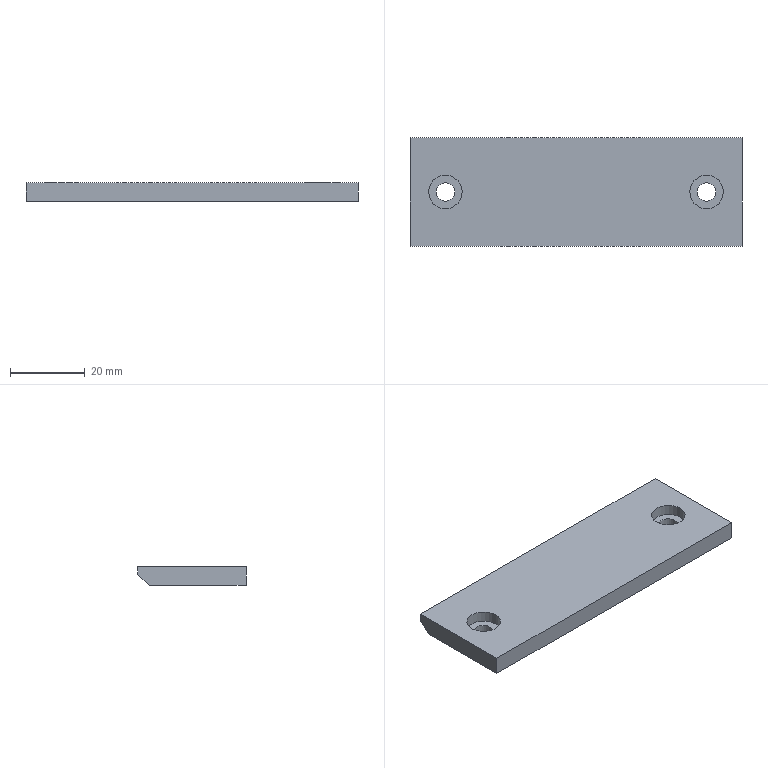Part | NX | features DATUM_CSYS 3, EXTRUDE 3, SKETCH 2 | 1 solid | 13 faces | box 89 x 29 x 5 mm | volume 12044 mm3 | plane 9 | cylinder 4 | commonest cylinder face diameters 5 x2 9 x2
STEP:
#1=CARTESIAN_POINT('',(0.,26.,0.));
#2=VERTEX_POINT('',#1);
#3=CARTESIAN_POINT('',(0.,29.,3.));
#4=VERTEX_POINT('',#3);
#5=CARTESIAN_POINT('',(0.,26.,0.));
#6=DIRECTION('',(0.,0.7071,0.7071));
#7=VECTOR('',#6,1000.);
#8=LINE('',#5,#7);
#9=EDGE_CURVE('',#2,#4,#8,.T.);
#10=ORIENTED_EDGE('',*,*,#9,.F.);
#11=CARTESIAN_POINT('',(0.,0.,0.));
#12=VERTEX_POINT('',#11);
#13=CARTESIAN_POINT('',(0.,29.,0.));
#14=DIRECTION('',(0.,-1.,0.));
#15=VECTOR('',#14,1000.);
#16=LINE('',#13,#15);
#17=EDGE_CURVE('',#2,#12,#16,.T.);
#18=ORIENTED_EDGE('',*,*,#17,.T.);
#19=CARTESIAN_POINT('',(0.,0.,5.));
#20=VERTEX_POINT('',#19);
#21=CARTESIAN_POINT('',(0.,0.,5.));
#22=DIRECTION('',(0.,0.,-1.));
#23=VECTOR('',#22,1000.);
#24=LINE('',#21,#23);
#25=EDGE_CURVE('',#20,#12,#24,.T.);
#26=ORIENTED_EDGE('',*,*,#25,.F.);
#27=CARTESIAN_POINT('',(0.,29.,5.));
#28=VERTEX_POINT('',#27);
#29=CARTESIAN_POINT('',(0.,29.,5.));
#30=DIRECTION('',(0.,-1.,0.));
#31=VECTOR('',#30,1000.);
#32=LINE('',#29,#31);
#33=EDGE_CURVE('',#28,#20,#32,.T.);
#34=ORIENTED_EDGE('',*,*,#33,.F.);
#35=CARTESIAN_POINT('',(0.,29.,5.));
#36=DIRECTION('',(0.,0.,-1.));
#37=VECTOR('',#36,1000.);
#38=LINE('',#35,#37);
#39=EDGE_CURVE('',#28,#4,#38,.T.);
#40=ORIENTED_EDGE('',*,*,#39,.T.);
#41=EDGE_LOOP('',(#10,#18,#26,#34,#40));
#42=FACE_BOUND('',#41,.T.);
#43=CARTESIAN_POINT('',(0.,29.,5.));
#44=DIRECTION('',(1.,0.,0.));
#45=DIRECTION('',(0.,0.,-1.));
#46=AXIS2_PLACEMENT_3D('',#43,#44,#45);
#47=PLANE('',#46);
#48=ADVANCED_FACE('',(#42),#47,.F.);
#49=CARTESIAN_POINT('',(75.,14.5,5.));
#50=VERTEX_POINT('',#49);
#51=CARTESIAN_POINT('',(79.5,14.5,5.));
#52=DIRECTION('',(0.,0.,-1.));
#53=DIRECTION('',(-1.,0.,0.));
#54=AXIS2_PLACEMENT_3D('',#51,#52,#53);
#55=CIRCLE('',#54,4.5);
#56=EDGE_CURVE('',#50,#50,#55,.T.);
#57=ORIENTED_EDGE('',*,*,#56,.F.);
#58=EDGE_LOOP('',(#57));
#59=FACE_BOUND('',#58,.T.);
#60=CARTESIAN_POINT('',(75.,14.5,2.));
#61=VERTEX_POINT('',#60);
#62=CARTESIAN_POINT('',(79.5,14.5,2.));
#63=DIRECTION('',(0.,0.,-1.));
#64=DIRECTION('',(-1.,0.,0.));
#65=AXIS2_PLACEMENT_3D('',#62,#63,#64);
#66=CIRCLE('',#65,4.5);
#67=EDGE_CURVE('',#61,#61,#66,.F.);
#68=ORIENTED_EDGE('',*,*,#67,.F.);
#69=EDGE_LOOP('',(#68));
#70=FACE_BOUND('',#69,.T.);
#71=CARTESIAN_POINT('',(79.5,14.5,5.));
#72=DIRECTION('',(0.,0.,-1.));
#73=DIRECTION('',(-1.,0.,0.));
#74=AXIS2_PLACEMENT_3D('',#71,#72,#73);
#75=CYLINDRICAL_SURFACE('',#74,4.5);
#76=ADVANCED_FACE('',(#59,#70),#75,.F.);
#77=CARTESIAN_POINT('',(89.,0.,0.));
#78=VERTEX_POINT('',#77);
#79=CARTESIAN_POINT('',(0.,0.,0.));
#80=DIRECTION('',(1.,0.,0.));
#81=VECTOR('',#80,1000.);
#82=LINE('',#79,#81);
#83=EDGE_CURVE('',#12,#78,#82,.T.);
#84=ORIENTED_EDGE('',*,*,#83,.T.);
#85=CARTESIAN_POINT('',(89.,0.,5.));
#86=VERTEX_POINT('',#85);
#87=CARTESIAN_POINT('',(89.,0.,5.));
#88=DIRECTION('',(0.,0.,-1.));
#89=VECTOR('',#88,1000.);
#90=LINE('',#87,#89);
#91=EDGE_CURVE('',#86,#78,#90,.T.);
#92=ORIENTED_EDGE('',*,*,#91,.F.);
#93=CARTESIAN_POINT('',(0.,0.,5.));
#94=DIRECTION('',(1.,0.,0.));
#95=VECTOR('',#94,1000.);
#96=LINE('',#93,#95);
#97=EDGE_CURVE('',#20,#86,#96,.T.);
#98=ORIENTED_EDGE('',*,*,#97,.F.);
#99=ORIENTED_EDGE('',*,*,#25,.T.);
#100=EDGE_LOOP('',(#84,#92,#98,#99));
#101=FACE_BOUND('',#100,.T.);
#102=CARTESIAN_POINT('',(0.,0.,5.));
#103=DIRECTION('',(0.,1.,0.));
#104=DIRECTION('',(0.,0.,1.));
#105=AXIS2_PLACEMENT_3D('',#102,#103,#104);
#106=PLANE('',#105);
#107=ADVANCED_FACE('',(#101),#106,.F.);
#108=CARTESIAN_POINT('',(89.,26.,0.));
#109=VERTEX_POINT('',#108);
#110=CARTESIAN_POINT('',(89.,0.,0.));
#111=DIRECTION('',(0.,1.,0.));
#112=VECTOR('',#111,1000.);
#113=LINE('',#110,#112);
#114=EDGE_CURVE('',#78,#109,#113,.T.);
#115=ORIENTED_EDGE('',*,*,#114,.T.);
#116=CARTESIAN_POINT('',(89.,29.,3.));
#117=VERTEX_POINT('',#116);
#118=CARTESIAN_POINT('',(89.,15.5,-10.5));
#119=DIRECTION('',(0.,0.7071,0.7071));
#120=VECTOR('',#119,1000.);
#121=LINE('',#118,#120);
#122=EDGE_CURVE('',#109,#117,#121,.T.);
#123=ORIENTED_EDGE('',*,*,#122,.T.);
#124=CARTESIAN_POINT('',(89.,29.,5.));
#125=VERTEX_POINT('',#124);
#126=CARTESIAN_POINT('',(89.,29.,5.));
#127=DIRECTION('',(0.,0.,-1.));
#128=VECTOR('',#127,1000.);
#129=LINE('',#126,#128);
#130=EDGE_CURVE('',#125,#117,#129,.T.);
#131=ORIENTED_EDGE('',*,*,#130,.F.);
#132=CARTESIAN_POINT('',(89.,0.,5.));
#133=DIRECTION('',(0.,1.,0.));
#134=VECTOR('',#133,1000.);
#135=LINE('',#132,#134);
#136=EDGE_CURVE('',#86,#125,#135,.T.);
#137=ORIENTED_EDGE('',*,*,#136,.F.);
#138=ORIENTED_EDGE('',*,*,#91,.T.);
#139=EDGE_LOOP('',(#115,#123,#131,#137,#138));
#140=FACE_BOUND('',#139,.T.);
#141=CARTESIAN_POINT('',(89.,0.,5.));
#142=DIRECTION('',(-1.,0.,0.));
#143=DIRECTION('',(0.,0.,1.));
#144=AXIS2_PLACEMENT_3D('',#141,#142,#143);
#145=PLANE('',#144);
#146=ADVANCED_FACE('',(#140),#145,.F.);
#147=ORIENTED_EDGE('',*,*,#130,.T.);
#148=CARTESIAN_POINT('',(55000.,29.,3.));
#149=DIRECTION('',(-1.,0.,0.));
#150=VECTOR('',#149,1000.);
#151=LINE('',#148,#150);
#152=EDGE_CURVE('',#117,#4,#151,.T.);
#153=ORIENTED_EDGE('',*,*,#152,.T.);
#154=ORIENTED_EDGE('',*,*,#39,.F.);
#155=CARTESIAN_POINT('',(89.,29.,5.));
#156=DIRECTION('',(-1.,0.,0.));
#157=VECTOR('',#156,1000.);
#158=LINE('',#155,#157);
#159=EDGE_CURVE('',#125,#28,#158,.T.);
#160=ORIENTED_EDGE('',*,*,#159,.F.);
#161=EDGE_LOOP('',(#147,#153,#154,#160));
#162=FACE_BOUND('',#161,.T.);
#163=CARTESIAN_POINT('',(89.,29.,5.));
#164=DIRECTION('',(0.,-1.,0.));
#165=DIRECTION('',(1.,0.,0.));
#166=AXIS2_PLACEMENT_3D('',#163,#164,#165);
#167=PLANE('',#166);
#168=ADVANCED_FACE('',(#162),#167,.F.);
#169=CARTESIAN_POINT('',(14.,14.5,2.));
#170=VERTEX_POINT('',#169);
#171=CARTESIAN_POINT('',(9.5,14.5,2.));
#172=DIRECTION('',(0.,0.,1.));
#173=DIRECTION('',(1.,0.,0.));
#174=AXIS2_PLACEMENT_3D('',#171,#172,#173);
#175=CIRCLE('',#174,4.5);
#176=EDGE_CURVE('',#170,#170,#175,.T.);
#177=ORIENTED_EDGE('',*,*,#176,.F.);
#178=EDGE_LOOP('',(#177));
#179=FACE_BOUND('',#178,.T.);
#180=CARTESIAN_POINT('',(14.,14.5,5.));
#181=VERTEX_POINT('',#180);
#182=CARTESIAN_POINT('',(9.5,14.5,5.));
#183=DIRECTION('',(0.,0.,1.));
#184=DIRECTION('',(1.,0.,0.));
#185=AXIS2_PLACEMENT_3D('',#182,#183,#184);
#186=CIRCLE('',#185,4.5);
#187=EDGE_CURVE('',#181,#181,#186,.T.);
#188=ORIENTED_EDGE('',*,*,#187,.T.);
#189=EDGE_LOOP('',(#188));
#190=FACE_BOUND('',#189,.T.);
#191=CARTESIAN_POINT('',(9.5,14.5,5.));
#192=DIRECTION('',(0.,0.,-1.));
#193=DIRECTION('',(-1.,0.,0.));
#194=AXIS2_PLACEMENT_3D('',#191,#192,#193);
#195=CYLINDRICAL_SURFACE('',#194,4.5);
#196=ADVANCED_FACE('',(#179,#190),#195,.F.);
#197=ORIENTED_EDGE('',*,*,#33,.T.);
#198=ORIENTED_EDGE('',*,*,#97,.T.);
#199=ORIENTED_EDGE('',*,*,#136,.T.);
#200=ORIENTED_EDGE('',*,*,#159,.T.);
#201=EDGE_LOOP('',(#197,#198,#199,#200));
#202=FACE_BOUND('',#201,.T.);
#203=ORIENTED_EDGE('',*,*,#56,.T.);
#204=EDGE_LOOP('',(#203));
#205=FACE_BOUND('',#204,.T.);
#206=ORIENTED_EDGE('',*,*,#187,.F.);
#207=EDGE_LOOP('',(#206));
#208=FACE_BOUND('',#207,.T.);
#209=CARTESIAN_POINT('',(79.5,14.5,5.));
#210=DIRECTION('',(0.,0.,-1.));
#211=DIRECTION('',(-1.,0.,0.));
#212=AXIS2_PLACEMENT_3D('',#209,#210,#211);
#213=PLANE('',#212);
#214=ADVANCED_FACE('',(#202,#205,#208),#213,.F.);
#215=CARTESIAN_POINT('',(55000.,26.,0.));
#216=DIRECTION('',(-1.,0.,0.));
#217=VECTOR('',#216,1000.);
#218=LINE('',#215,#217);
#219=EDGE_CURVE('',#109,#2,#218,.T.);
#220=ORIENTED_EDGE('',*,*,#219,.F.);
#221=ORIENTED_EDGE('',*,*,#114,.F.);
#222=ORIENTED_EDGE('',*,*,#83,.F.);
#223=ORIENTED_EDGE('',*,*,#17,.F.);
#224=EDGE_LOOP('',(#220,#221,#222,#223));
#225=FACE_BOUND('',#224,.T.);
#226=CARTESIAN_POINT('',(12.,14.5,0.));
#227=VERTEX_POINT('',#226);
#228=CARTESIAN_POINT('',(9.5,14.5,0.));
#229=DIRECTION('',(0.,0.,1.));
#230=DIRECTION('',(1.,0.,0.));
#231=AXIS2_PLACEMENT_3D('',#228,#229,#230);
#232=CIRCLE('',#231,2.5);
#233=EDGE_CURVE('',#227,#227,#232,.T.);
#234=ORIENTED_EDGE('',*,*,#233,.T.);
#235=EDGE_LOOP('',(#234));
#236=FACE_BOUND('',#235,.T.);
#237=CARTESIAN_POINT('',(77.,14.5,0.));
#238=VERTEX_POINT('',#237);
#239=CARTESIAN_POINT('',(79.5,14.5,0.));
#240=DIRECTION('',(0.,0.,-1.));
#241=DIRECTION('',(-1.,0.,0.));
#242=AXIS2_PLACEMENT_3D('',#239,#240,#241);
#243=CIRCLE('',#242,2.5);
#244=EDGE_CURVE('',#238,#238,#243,.T.);
#245=ORIENTED_EDGE('',*,*,#244,.F.);
#246=EDGE_LOOP('',(#245));
#247=FACE_BOUND('',#246,.T.);
#248=CARTESIAN_POINT('',(79.5,14.5,0.));
#249=DIRECTION('',(0.,0.,-1.));
#250=DIRECTION('',(-1.,0.,0.));
#251=AXIS2_PLACEMENT_3D('',#248,#249,#250);
#252=PLANE('',#251);
#253=ADVANCED_FACE('',(#225,#236,#247),#252,.T.);
#254=CARTESIAN_POINT('',(12.,14.5,2.));
#255=VERTEX_POINT('',#254);
#256=CARTESIAN_POINT('',(9.5,14.5,2.));
#257=DIRECTION('',(0.,0.,1.));
#258=DIRECTION('',(1.,0.,0.));
#259=AXIS2_PLACEMENT_3D('',#256,#257,#258);
#260=CIRCLE('',#259,2.5);
#261=EDGE_CURVE('',#255,#255,#260,.T.);
#262=ORIENTED_EDGE('',*,*,#261,.T.);
#263=EDGE_LOOP('',(#262));
#264=FACE_BOUND('',#263,.T.);
#265=ORIENTED_EDGE('',*,*,#233,.F.);
#266=EDGE_LOOP('',(#265));
#267=FACE_BOUND('',#266,.T.);
#268=CARTESIAN_POINT('',(9.5,14.5,2.));
#269=DIRECTION('',(0.,0.,-1.));
#270=DIRECTION('',(-1.,0.,0.));
#271=AXIS2_PLACEMENT_3D('',#268,#269,#270);
#272=CYLINDRICAL_SURFACE('',#271,2.5);
#273=ADVANCED_FACE('',(#264,#267),#272,.F.);
#274=ORIENTED_EDGE('',*,*,#176,.T.);
#275=EDGE_LOOP('',(#274));
#276=FACE_BOUND('',#275,.T.);
#277=ORIENTED_EDGE('',*,*,#261,.F.);
#278=EDGE_LOOP('',(#277));
#279=FACE_BOUND('',#278,.T.);
#280=CARTESIAN_POINT('',(9.5,14.5,2.));
#281=DIRECTION('',(0.,0.,1.));
#282=DIRECTION('',(1.,0.,0.));
#283=AXIS2_PLACEMENT_3D('',#280,#281,#282);
#284=PLANE('',#283);
#285=ADVANCED_FACE('',(#276,#279),#284,.T.);
#286=CARTESIAN_POINT('',(77.,14.5,2.));
#287=VERTEX_POINT('',#286);
#288=CARTESIAN_POINT('',(79.5,14.5,2.));
#289=DIRECTION('',(0.,0.,-1.));
#290=DIRECTION('',(-1.,0.,0.));
#291=AXIS2_PLACEMENT_3D('',#288,#289,#290);
#292=CIRCLE('',#291,2.5);
#293=EDGE_CURVE('',#287,#287,#292,.T.);
#294=ORIENTED_EDGE('',*,*,#293,.F.);
#295=EDGE_LOOP('',(#294));
#296=FACE_BOUND('',#295,.T.);
#297=ORIENTED_EDGE('',*,*,#244,.T.);
#298=EDGE_LOOP('',(#297));
#299=FACE_BOUND('',#298,.T.);
#300=CARTESIAN_POINT('',(79.5,14.5,2.));
#301=DIRECTION('',(0.,0.,-1.));
#302=DIRECTION('',(-1.,0.,0.));
#303=AXIS2_PLACEMENT_3D('',#300,#301,#302);
#304=CYLINDRICAL_SURFACE('',#303,2.5);
#305=ADVANCED_FACE('',(#296,#299),#304,.F.);
#306=ORIENTED_EDGE('',*,*,#67,.T.);
#307=EDGE_LOOP('',(#306));
#308=FACE_BOUND('',#307,.T.);
#309=ORIENTED_EDGE('',*,*,#293,.T.);
#310=EDGE_LOOP('',(#309));
#311=FACE_BOUND('',#310,.T.);
#312=CARTESIAN_POINT('',(79.5,14.5,2.));
#313=DIRECTION('',(0.,0.,-1.));
#314=DIRECTION('',(-1.,0.,0.));
#315=AXIS2_PLACEMENT_3D('',#312,#313,#314);
#316=PLANE('',#315);
#317=ADVANCED_FACE('',(#308,#311),#316,.F.);
#318=ORIENTED_EDGE('',*,*,#219,.T.);
#319=ORIENTED_EDGE('',*,*,#9,.T.);
#320=ORIENTED_EDGE('',*,*,#152,.F.);
#321=ORIENTED_EDGE('',*,*,#122,.F.);
#322=EDGE_LOOP('',(#318,#319,#320,#321));
#323=FACE_BOUND('',#322,.T.);
#324=CARTESIAN_POINT('',(55000.,26.,0.));
#325=DIRECTION('',(0.,-0.7071,0.7071));
#326=DIRECTION('',(0.,-0.7071,-0.7071));
#327=AXIS2_PLACEMENT_3D('',#324,#325,#326);
#328=PLANE('',#327);
#329=ADVANCED_FACE('',(#323),#328,.F.);
#330=CLOSED_SHELL('',(#48,#76,#107,#146,#168,#196,#214,#253,#273,#285,#305,#317,#329));
#331=MANIFOLD_SOLID_BREP('',#330);
#332=(LENGTH_UNIT()NAMED_UNIT(*)SI_UNIT(.MILLI.,.METRE.));
#333=UNCERTAINTY_MEASURE_WITH_UNIT(LENGTH_MEASURE(0.00001),#332,'','');
#334=(NAMED_UNIT(*)PLANE_ANGLE_UNIT()SI_UNIT($,.RADIAN.));
#335=(NAMED_UNIT(*)SI_UNIT($,.STERADIAN.)SOLID_ANGLE_UNIT());
#336=(GEOMETRIC_REPRESENTATION_CONTEXT(3)GLOBAL_UNCERTAINTY_ASSIGNED_CONTEXT((#333))GLOBAL_UNIT_ASSIGNED_CONTEXT((#332,#334,#335))REPRESENTATION_CONTEXT('',''));
#337=ADVANCED_BREP_SHAPE_REPRESENTATION('',(#331),#336);